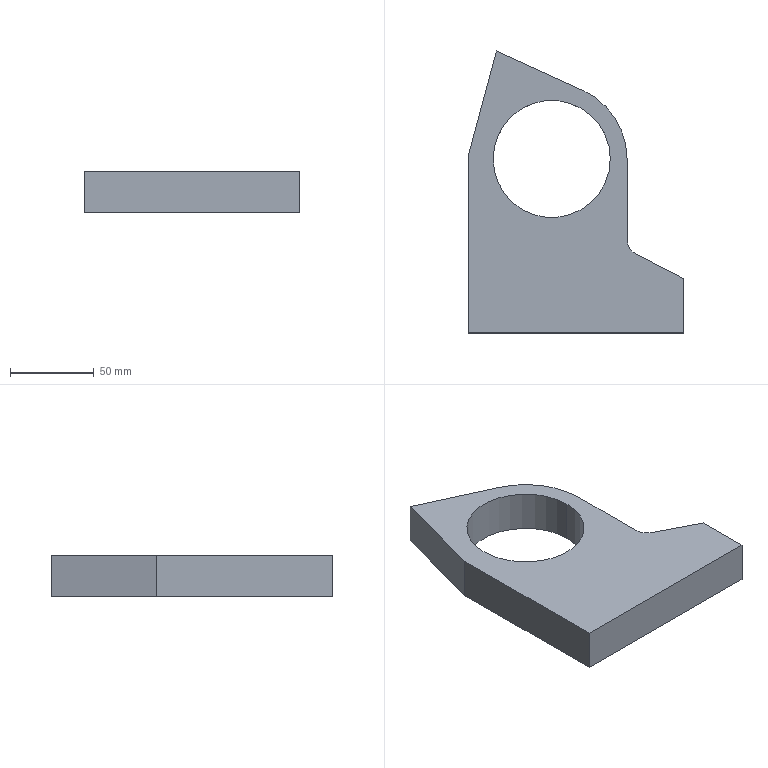Part | SolidWorks | features Extrusion 1 | 1 solid | 13 faces | box 129 x 168.47 x 25 mm | volume 287390 mm3 | plane 9 | cylinder 4 | commonest cylinder face diameters 70 x2 20 x1 90 x1
STEP:
#1=CARTESIAN_POINT('',(15.,81.5,25.));
#2=VERTEX_POINT('',#1);
#3=CARTESIAN_POINT('',(85.,81.5,25.));
#4=VERTEX_POINT('',#3);
#5=CARTESIAN_POINT('',(50.,81.5,25.));
#6=DIRECTION('',(0.,0.,1.));
#7=DIRECTION('',(1.,0.,0.));
#8=AXIS2_PLACEMENT_3D('',#5,#6,#7);
#9=CIRCLE('',#8,35.);
#10=EDGE_CURVE('',#2,#4,#9,.T.);
#11=ORIENTED_EDGE('',*,*,#10,.T.);
#12=CARTESIAN_POINT('',(85.,81.5,0.));
#13=VERTEX_POINT('',#12);
#14=CARTESIAN_POINT('',(85.,81.5,25.));
#15=DIRECTION('',(0.,0.,-1.));
#16=VECTOR('',#15,1000.);
#17=LINE('',#14,#16);
#18=EDGE_CURVE('',#4,#13,#17,.T.);
#19=ORIENTED_EDGE('',*,*,#18,.T.);
#20=CARTESIAN_POINT('',(15.,81.5,0.));
#21=VERTEX_POINT('',#20);
#22=CARTESIAN_POINT('',(50.,81.5,0.));
#23=DIRECTION('',(0.,0.,1.));
#24=DIRECTION('',(1.,0.,0.));
#25=AXIS2_PLACEMENT_3D('',#22,#23,#24);
#26=CIRCLE('',#25,35.);
#27=EDGE_CURVE('',#21,#13,#26,.T.);
#28=ORIENTED_EDGE('',*,*,#27,.F.);
#29=CARTESIAN_POINT('',(15.,81.5,25.));
#30=DIRECTION('',(0.,0.,-1.));
#31=VECTOR('',#30,1000.);
#32=LINE('',#29,#31);
#33=EDGE_CURVE('',#2,#21,#32,.T.);
#34=ORIENTED_EDGE('',*,*,#33,.F.);
#35=EDGE_LOOP('',(#11,#19,#28,#34));
#36=FACE_OUTER_BOUND('',#35,.T.);
#37=CARTESIAN_POINT('',(50.,81.5,25.));
#38=DIRECTION('',(0.,0.,-1.));
#39=DIRECTION('',(-1.,0.,0.));
#40=AXIS2_PLACEMENT_3D('',#37,#38,#39);
#41=CYLINDRICAL_SURFACE('',#40,35.);
#42=ADVANCED_FACE('',(#36),#41,.F.);
#43=CARTESIAN_POINT('',(0.,-22.47,25.));
#44=VERTEX_POINT('',#43);
#45=CARTESIAN_POINT('',(129.,-22.47,25.));
#46=VERTEX_POINT('',#45);
#47=CARTESIAN_POINT('',(129.,-22.47,25.));
#48=DIRECTION('',(1.,0.,0.));
#49=VECTOR('',#48,1000.);
#50=LINE('',#47,#49);
#51=EDGE_CURVE('',#44,#46,#50,.T.);
#52=ORIENTED_EDGE('',*,*,#51,.T.);
#53=CARTESIAN_POINT('',(129.,10.,25.));
#54=VERTEX_POINT('',#53);
#55=CARTESIAN_POINT('',(129.,0.,25.));
#56=DIRECTION('',(0.,1.,0.));
#57=VECTOR('',#56,1000.);
#58=LINE('',#55,#57);
#59=EDGE_CURVE('',#46,#54,#58,.T.);
#60=ORIENTED_EDGE('',*,*,#59,.T.);
#61=CARTESIAN_POINT('',(100.448,24.596,25.));
#62=VERTEX_POINT('',#61);
#63=CARTESIAN_POINT('',(129.,10.,25.));
#64=DIRECTION('',(-0.8904,0.4552,0.));
#65=VECTOR('',#64,1000.);
#66=LINE('',#63,#65);
#67=EDGE_CURVE('',#54,#62,#66,.T.);
#68=ORIENTED_EDGE('',*,*,#67,.T.);
#69=CARTESIAN_POINT('',(95.,33.5,25.));
#70=VERTEX_POINT('',#69);
#71=CARTESIAN_POINT('',(105.,33.5,25.));
#72=DIRECTION('',(0.,0.,-1.));
#73=DIRECTION('',(1.,0.,0.));
#74=AXIS2_PLACEMENT_3D('',#71,#72,#73);
#75=CIRCLE('',#74,10.);
#76=EDGE_CURVE('',#62,#70,#75,.T.);
#77=ORIENTED_EDGE('',*,*,#76,.T.);
#78=CARTESIAN_POINT('',(95.,81.5,25.));
#79=VERTEX_POINT('',#78);
#80=CARTESIAN_POINT('',(95.,81.5,25.));
#81=DIRECTION('',(0.,1.,0.));
#82=VECTOR('',#81,1000.);
#83=LINE('',#80,#82);
#84=EDGE_CURVE('',#70,#79,#83,.T.);
#85=ORIENTED_EDGE('',*,*,#84,.T.);
#86=CARTESIAN_POINT('',(68.639,122.458,25.));
#87=VERTEX_POINT('',#86);
#88=CARTESIAN_POINT('',(50.,81.5,25.));
#89=DIRECTION('',(0.,0.,1.));
#90=DIRECTION('',(1.,0.,0.));
#91=AXIS2_PLACEMENT_3D('',#88,#89,#90);
#92=CIRCLE('',#91,45.);
#93=EDGE_CURVE('',#79,#87,#92,.T.);
#94=ORIENTED_EDGE('',*,*,#93,.T.);
#95=CARTESIAN_POINT('',(16.908,146.,25.));
#96=VERTEX_POINT('',#95);
#97=CARTESIAN_POINT('',(16.908,146.,25.));
#98=DIRECTION('',(-0.9102,0.4142,0.));
#99=VECTOR('',#98,1000.);
#100=LINE('',#97,#99);
#101=EDGE_CURVE('',#87,#96,#100,.T.);
#102=ORIENTED_EDGE('',*,*,#101,.T.);
#103=CARTESIAN_POINT('',(0.,82.9,25.));
#104=VERTEX_POINT('',#103);
#105=CARTESIAN_POINT('',(16.908,146.,25.));
#106=DIRECTION('',(-0.2588,-0.9659,0.));
#107=VECTOR('',#106,1000.);
#108=LINE('',#105,#107);
#109=EDGE_CURVE('',#96,#104,#108,.T.);
#110=ORIENTED_EDGE('',*,*,#109,.T.);
#111=CARTESIAN_POINT('',(0.,-22.47,25.));
#112=DIRECTION('',(0.,-1.,0.));
#113=VECTOR('',#112,1000.);
#114=LINE('',#111,#113);
#115=EDGE_CURVE('',#104,#44,#114,.T.);
#116=ORIENTED_EDGE('',*,*,#115,.T.);
#117=EDGE_LOOP('',(#52,#60,#68,#77,#85,#94,#102,#110,#116));
#118=FACE_OUTER_BOUND('',#117,.T.);
#119=ORIENTED_EDGE('',*,*,#10,.F.);
#120=CARTESIAN_POINT('',(50.,81.5,25.));
#121=DIRECTION('',(0.,0.,1.));
#122=DIRECTION('',(1.,0.,0.));
#123=AXIS2_PLACEMENT_3D('',#120,#121,#122);
#124=CIRCLE('',#123,35.);
#125=EDGE_CURVE('',#4,#2,#124,.T.);
#126=ORIENTED_EDGE('',*,*,#125,.F.);
#127=EDGE_LOOP('',(#119,#126));
#128=FACE_BOUND('',#127,.T.);
#129=CARTESIAN_POINT('',(50.,81.5,25.));
#130=DIRECTION('',(0.,0.,1.));
#131=DIRECTION('',(1.,0.,0.));
#132=AXIS2_PLACEMENT_3D('',#129,#130,#131);
#133=PLANE('',#132);
#134=ADVANCED_FACE('',(#118,#128),#133,.T.);
#135=CARTESIAN_POINT('',(0.,-22.47,0.));
#136=VERTEX_POINT('',#135);
#137=CARTESIAN_POINT('',(129.,-22.47,0.));
#138=VERTEX_POINT('',#137);
#139=CARTESIAN_POINT('',(129.,-22.47,0.));
#140=DIRECTION('',(1.,0.,0.));
#141=VECTOR('',#140,1000.);
#142=LINE('',#139,#141);
#143=EDGE_CURVE('',#136,#138,#142,.T.);
#144=ORIENTED_EDGE('',*,*,#143,.F.);
#145=CARTESIAN_POINT('',(0.,82.9,0.));
#146=VERTEX_POINT('',#145);
#147=CARTESIAN_POINT('',(0.,-22.47,0.));
#148=DIRECTION('',(0.,-1.,0.));
#149=VECTOR('',#148,1000.);
#150=LINE('',#147,#149);
#151=EDGE_CURVE('',#146,#136,#150,.T.);
#152=ORIENTED_EDGE('',*,*,#151,.F.);
#153=CARTESIAN_POINT('',(16.908,146.,0.));
#154=VERTEX_POINT('',#153);
#155=CARTESIAN_POINT('',(16.908,146.,0.));
#156=DIRECTION('',(-0.2588,-0.9659,0.));
#157=VECTOR('',#156,1000.);
#158=LINE('',#155,#157);
#159=EDGE_CURVE('',#154,#146,#158,.T.);
#160=ORIENTED_EDGE('',*,*,#159,.F.);
#161=CARTESIAN_POINT('',(68.639,122.458,0.));
#162=VERTEX_POINT('',#161);
#163=CARTESIAN_POINT('',(16.908,146.,0.));
#164=DIRECTION('',(-0.9102,0.4142,0.));
#165=VECTOR('',#164,1000.);
#166=LINE('',#163,#165);
#167=EDGE_CURVE('',#162,#154,#166,.T.);
#168=ORIENTED_EDGE('',*,*,#167,.F.);
#169=CARTESIAN_POINT('',(95.,81.5,0.));
#170=VERTEX_POINT('',#169);
#171=CARTESIAN_POINT('',(50.,81.5,0.));
#172=DIRECTION('',(0.,0.,1.));
#173=DIRECTION('',(1.,0.,0.));
#174=AXIS2_PLACEMENT_3D('',#171,#172,#173);
#175=CIRCLE('',#174,45.);
#176=EDGE_CURVE('',#170,#162,#175,.T.);
#177=ORIENTED_EDGE('',*,*,#176,.F.);
#178=CARTESIAN_POINT('',(95.,33.5,0.));
#179=VERTEX_POINT('',#178);
#180=CARTESIAN_POINT('',(95.,81.5,0.));
#181=DIRECTION('',(0.,1.,0.));
#182=VECTOR('',#181,1000.);
#183=LINE('',#180,#182);
#184=EDGE_CURVE('',#179,#170,#183,.T.);
#185=ORIENTED_EDGE('',*,*,#184,.F.);
#186=CARTESIAN_POINT('',(100.448,24.596,0.));
#187=VERTEX_POINT('',#186);
#188=CARTESIAN_POINT('',(105.,33.5,0.));
#189=DIRECTION('',(0.,0.,-1.));
#190=DIRECTION('',(1.,0.,0.));
#191=AXIS2_PLACEMENT_3D('',#188,#189,#190);
#192=CIRCLE('',#191,10.);
#193=EDGE_CURVE('',#187,#179,#192,.T.);
#194=ORIENTED_EDGE('',*,*,#193,.F.);
#195=CARTESIAN_POINT('',(129.,10.,0.));
#196=VERTEX_POINT('',#195);
#197=CARTESIAN_POINT('',(129.,10.,0.));
#198=DIRECTION('',(-0.8904,0.4552,0.));
#199=VECTOR('',#198,1000.);
#200=LINE('',#197,#199);
#201=EDGE_CURVE('',#196,#187,#200,.T.);
#202=ORIENTED_EDGE('',*,*,#201,.F.);
#203=CARTESIAN_POINT('',(129.,0.,0.));
#204=DIRECTION('',(0.,1.,0.));
#205=VECTOR('',#204,1000.);
#206=LINE('',#203,#205);
#207=EDGE_CURVE('',#138,#196,#206,.T.);
#208=ORIENTED_EDGE('',*,*,#207,.F.);
#209=EDGE_LOOP('',(#144,#152,#160,#168,#177,#185,#194,#202,#208));
#210=FACE_OUTER_BOUND('',#209,.T.);
#211=ORIENTED_EDGE('',*,*,#27,.T.);
#212=CARTESIAN_POINT('',(50.,81.5,0.));
#213=DIRECTION('',(0.,0.,1.));
#214=DIRECTION('',(1.,0.,0.));
#215=AXIS2_PLACEMENT_3D('',#212,#213,#214);
#216=CIRCLE('',#215,35.);
#217=EDGE_CURVE('',#13,#21,#216,.T.);
#218=ORIENTED_EDGE('',*,*,#217,.T.);
#219=EDGE_LOOP('',(#211,#218));
#220=FACE_BOUND('',#219,.T.);
#221=CARTESIAN_POINT('',(50.,81.5,0.));
#222=DIRECTION('',(0.,0.,1.));
#223=DIRECTION('',(1.,0.,0.));
#224=AXIS2_PLACEMENT_3D('',#221,#222,#223);
#225=PLANE('',#224);
#226=ADVANCED_FACE('',(#210,#220),#225,.F.);
#227=ORIENTED_EDGE('',*,*,#143,.T.);
#228=CARTESIAN_POINT('',(129.,-22.47,25.));
#229=DIRECTION('',(0.,0.,-1.));
#230=VECTOR('',#229,1000.);
#231=LINE('',#228,#230);
#232=EDGE_CURVE('',#46,#138,#231,.T.);
#233=ORIENTED_EDGE('',*,*,#232,.F.);
#234=ORIENTED_EDGE('',*,*,#51,.F.);
#235=CARTESIAN_POINT('',(0.,-22.47,25.));
#236=DIRECTION('',(0.,0.,-1.));
#237=VECTOR('',#236,1000.);
#238=LINE('',#235,#237);
#239=EDGE_CURVE('',#44,#136,#238,.T.);
#240=ORIENTED_EDGE('',*,*,#239,.T.);
#241=EDGE_LOOP('',(#227,#233,#234,#240));
#242=FACE_OUTER_BOUND('',#241,.T.);
#243=CARTESIAN_POINT('',(129.,-22.47,25.));
#244=DIRECTION('',(0.,1.,0.));
#245=DIRECTION('',(-1.,0.,0.));
#246=AXIS2_PLACEMENT_3D('',#243,#244,#245);
#247=PLANE('',#246);
#248=ADVANCED_FACE('',(#242),#247,.F.);
#249=ORIENTED_EDGE('',*,*,#207,.T.);
#250=CARTESIAN_POINT('',(129.,10.,25.));
#251=DIRECTION('',(0.,0.,-1.));
#252=VECTOR('',#251,1000.);
#253=LINE('',#250,#252);
#254=EDGE_CURVE('',#54,#196,#253,.T.);
#255=ORIENTED_EDGE('',*,*,#254,.F.);
#256=ORIENTED_EDGE('',*,*,#59,.F.);
#257=ORIENTED_EDGE('',*,*,#232,.T.);
#258=EDGE_LOOP('',(#249,#255,#256,#257));
#259=FACE_OUTER_BOUND('',#258,.T.);
#260=CARTESIAN_POINT('',(129.,0.,25.));
#261=DIRECTION('',(-1.,0.,0.));
#262=DIRECTION('',(0.,-1.,0.));
#263=AXIS2_PLACEMENT_3D('',#260,#261,#262);
#264=PLANE('',#263);
#265=ADVANCED_FACE('',(#259),#264,.F.);
#266=ORIENTED_EDGE('',*,*,#201,.T.);
#267=CARTESIAN_POINT('',(100.448,24.596,25.));
#268=DIRECTION('',(0.,0.,-1.));
#269=VECTOR('',#268,1000.);
#270=LINE('',#267,#269);
#271=EDGE_CURVE('',#62,#187,#270,.T.);
#272=ORIENTED_EDGE('',*,*,#271,.F.);
#273=ORIENTED_EDGE('',*,*,#67,.F.);
#274=ORIENTED_EDGE('',*,*,#254,.T.);
#275=EDGE_LOOP('',(#266,#272,#273,#274));
#276=FACE_OUTER_BOUND('',#275,.T.);
#277=CARTESIAN_POINT('',(129.,10.,25.));
#278=DIRECTION('',(-0.4552,-0.8904,0.));
#279=DIRECTION('',(0.8904,-0.4552,0.));
#280=AXIS2_PLACEMENT_3D('',#277,#278,#279);
#281=PLANE('',#280);
#282=ADVANCED_FACE('',(#276),#281,.F.);
#283=ORIENTED_EDGE('',*,*,#193,.T.);
#284=CARTESIAN_POINT('',(95.,33.5,25.));
#285=DIRECTION('',(0.,0.,-1.));
#286=VECTOR('',#285,1000.);
#287=LINE('',#284,#286);
#288=EDGE_CURVE('',#70,#179,#287,.T.);
#289=ORIENTED_EDGE('',*,*,#288,.F.);
#290=ORIENTED_EDGE('',*,*,#76,.F.);
#291=ORIENTED_EDGE('',*,*,#271,.T.);
#292=EDGE_LOOP('',(#283,#289,#290,#291));
#293=FACE_OUTER_BOUND('',#292,.T.);
#294=CARTESIAN_POINT('',(105.,33.5,25.));
#295=DIRECTION('',(0.,0.,-1.));
#296=DIRECTION('',(-1.,0.,0.));
#297=AXIS2_PLACEMENT_3D('',#294,#295,#296);
#298=CYLINDRICAL_SURFACE('',#297,10.);
#299=ADVANCED_FACE('',(#293),#298,.F.);
#300=ORIENTED_EDGE('',*,*,#184,.T.);
#301=CARTESIAN_POINT('',(95.,81.5,25.));
#302=DIRECTION('',(0.,0.,-1.));
#303=VECTOR('',#302,1000.);
#304=LINE('',#301,#303);
#305=EDGE_CURVE('',#79,#170,#304,.T.);
#306=ORIENTED_EDGE('',*,*,#305,.F.);
#307=ORIENTED_EDGE('',*,*,#84,.F.);
#308=ORIENTED_EDGE('',*,*,#288,.T.);
#309=EDGE_LOOP('',(#300,#306,#307,#308));
#310=FACE_OUTER_BOUND('',#309,.T.);
#311=CARTESIAN_POINT('',(95.,81.5,25.));
#312=DIRECTION('',(-1.,0.,0.));
#313=DIRECTION('',(0.,0.,1.));
#314=AXIS2_PLACEMENT_3D('',#311,#312,#313);
#315=PLANE('',#314);
#316=ADVANCED_FACE('',(#310),#315,.F.);
#317=ORIENTED_EDGE('',*,*,#176,.T.);
#318=CARTESIAN_POINT('',(68.639,122.458,25.));
#319=DIRECTION('',(0.,0.,-1.));
#320=VECTOR('',#319,1000.);
#321=LINE('',#318,#320);
#322=EDGE_CURVE('',#87,#162,#321,.T.);
#323=ORIENTED_EDGE('',*,*,#322,.F.);
#324=ORIENTED_EDGE('',*,*,#93,.F.);
#325=ORIENTED_EDGE('',*,*,#305,.T.);
#326=EDGE_LOOP('',(#317,#323,#324,#325));
#327=FACE_OUTER_BOUND('',#326,.T.);
#328=CARTESIAN_POINT('',(50.,81.5,25.));
#329=DIRECTION('',(0.,0.,-1.));
#330=DIRECTION('',(-1.,0.,0.));
#331=AXIS2_PLACEMENT_3D('',#328,#329,#330);
#332=CYLINDRICAL_SURFACE('',#331,45.);
#333=ADVANCED_FACE('',(#327),#332,.T.);
#334=ORIENTED_EDGE('',*,*,#167,.T.);
#335=CARTESIAN_POINT('',(16.908,146.,25.));
#336=DIRECTION('',(0.,0.,-1.));
#337=VECTOR('',#336,1000.);
#338=LINE('',#335,#337);
#339=EDGE_CURVE('',#96,#154,#338,.T.);
#340=ORIENTED_EDGE('',*,*,#339,.F.);
#341=ORIENTED_EDGE('',*,*,#101,.F.);
#342=ORIENTED_EDGE('',*,*,#322,.T.);
#343=EDGE_LOOP('',(#334,#340,#341,#342));
#344=FACE_OUTER_BOUND('',#343,.T.);
#345=CARTESIAN_POINT('',(16.908,146.,25.));
#346=DIRECTION('',(-0.4142,-0.9102,0.));
#347=DIRECTION('',(0.9102,-0.4142,0.));
#348=AXIS2_PLACEMENT_3D('',#345,#346,#347);
#349=PLANE('',#348);
#350=ADVANCED_FACE('',(#344),#349,.F.);
#351=ORIENTED_EDGE('',*,*,#159,.T.);
#352=CARTESIAN_POINT('',(0.,82.9,25.));
#353=DIRECTION('',(0.,0.,-1.));
#354=VECTOR('',#353,1000.);
#355=LINE('',#352,#354);
#356=EDGE_CURVE('',#104,#146,#355,.T.);
#357=ORIENTED_EDGE('',*,*,#356,.F.);
#358=ORIENTED_EDGE('',*,*,#109,.F.);
#359=ORIENTED_EDGE('',*,*,#339,.T.);
#360=EDGE_LOOP('',(#351,#357,#358,#359));
#361=FACE_OUTER_BOUND('',#360,.T.);
#362=CARTESIAN_POINT('',(16.908,146.,25.));
#363=DIRECTION('',(0.9659,-0.2588,0.));
#364=DIRECTION('',(0.2588,0.9659,0.));
#365=AXIS2_PLACEMENT_3D('',#362,#363,#364);
#366=PLANE('',#365);
#367=ADVANCED_FACE('',(#361),#366,.F.);
#368=ORIENTED_EDGE('',*,*,#151,.T.);
#369=ORIENTED_EDGE('',*,*,#239,.F.);
#370=ORIENTED_EDGE('',*,*,#115,.F.);
#371=ORIENTED_EDGE('',*,*,#356,.T.);
#372=EDGE_LOOP('',(#368,#369,#370,#371));
#373=FACE_OUTER_BOUND('',#372,.T.);
#374=CARTESIAN_POINT('',(0.,-22.47,25.));
#375=DIRECTION('',(1.,0.,0.));
#376=DIRECTION('',(0.,1.,0.));
#377=AXIS2_PLACEMENT_3D('',#374,#375,#376);
#378=PLANE('',#377);
#379=ADVANCED_FACE('',(#373),#378,.F.);
#380=ORIENTED_EDGE('',*,*,#18,.F.);
#381=ORIENTED_EDGE('',*,*,#125,.T.);
#382=ORIENTED_EDGE('',*,*,#33,.T.);
#383=ORIENTED_EDGE('',*,*,#217,.F.);
#384=EDGE_LOOP('',(#380,#381,#382,#383));
#385=FACE_OUTER_BOUND('',#384,.T.);
#386=CARTESIAN_POINT('',(50.,81.5,25.));
#387=DIRECTION('',(0.,0.,-1.));
#388=DIRECTION('',(-1.,0.,0.));
#389=AXIS2_PLACEMENT_3D('',#386,#387,#388);
#390=CYLINDRICAL_SURFACE('',#389,35.);
#391=ADVANCED_FACE('',(#385),#390,.F.);
#392=CLOSED_SHELL('',(#42,#134,#226,#248,#265,#282,#299,#316,#333,#350,#367,#379,#391));
#393=MANIFOLD_SOLID_BREP('',#392);
#394=CARTESIAN_POINT('',(0.,0.,0.));
#395=DIRECTION('',(0.,0.,1.));
#396=DIRECTION('',(1.,0.,0.));
#397=AXIS2_PLACEMENT_3D('',#394,#395,#396);
#398=(LENGTH_UNIT()NAMED_UNIT(*)SI_UNIT(.MILLI.,.METRE.));
#399=UNCERTAINTY_MEASURE_WITH_UNIT(LENGTH_MEASURE(0.00001),#398,'','');
#400=(NAMED_UNIT(*)PLANE_ANGLE_UNIT()SI_UNIT($,.RADIAN.));
#401=(NAMED_UNIT(*)SI_UNIT($,.STERADIAN.)SOLID_ANGLE_UNIT());
#402=(GEOMETRIC_REPRESENTATION_CONTEXT(3)GLOBAL_UNCERTAINTY_ASSIGNED_CONTEXT((#399))GLOBAL_UNIT_ASSIGNED_CONTEXT((#398,#400,#401))REPRESENTATION_CONTEXT('',''));
#403=ADVANCED_BREP_SHAPE_REPRESENTATION('',(#393,#397),#402);